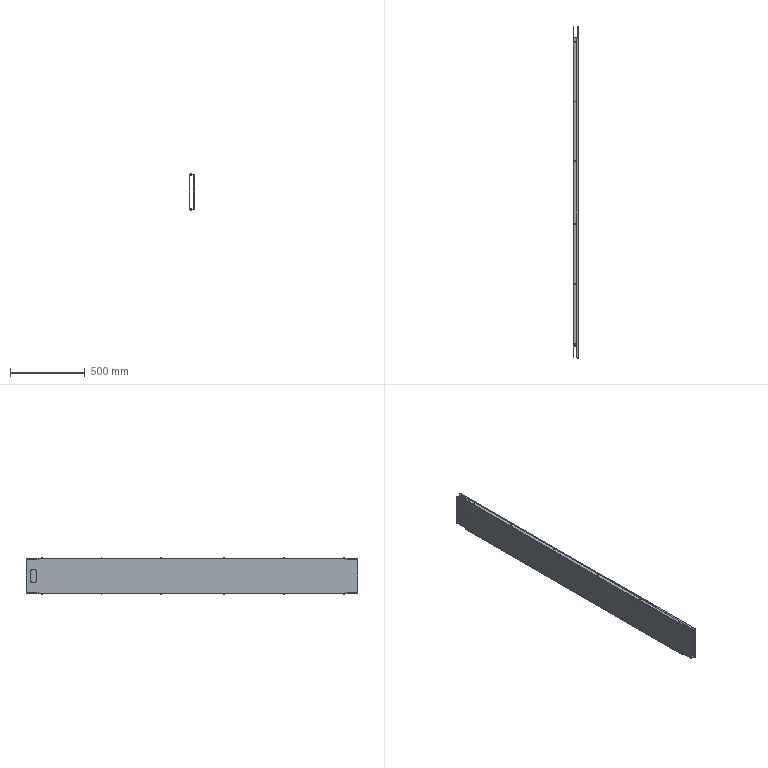Part | SolidWorks | features ReferencePattern 7, MirrorCompFeat 2 | 16 solids | 303 faces | box 36 x 2216 x 253 mm | volume 1745634 mm3 | plane 164 | cylinder 139 | commonest cylinder face diameters 6 x32 6.2 x24 8 x24 8.2 x24 12 x24 0.4 x4